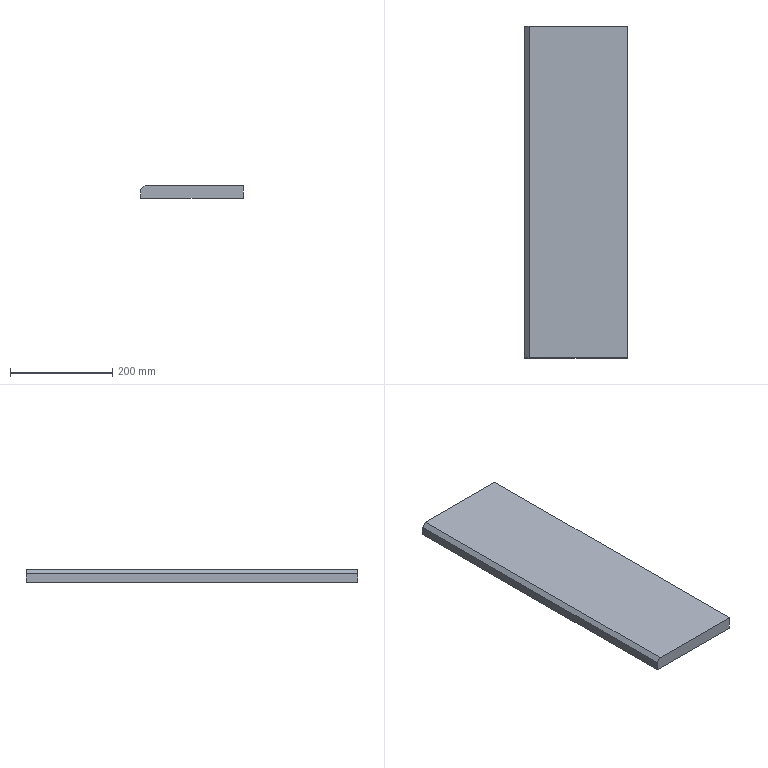Part | SolidWorks | features Chamfer 1, Extrusion 1 | 1 solid | 7 faces | box 200 x 650 x 25 mm | volume 3229200 mm3 | plane 7
STEP:
#1=CARTESIAN_POINT('',(0.,0.,17.));
#2=VERTEX_POINT('',#1);
#3=CARTESIAN_POINT('',(0.,0.,0.));
#4=VERTEX_POINT('',#3);
#5=CARTESIAN_POINT('',(0.,0.,25.));
#6=DIRECTION('',(0.,0.,-1.));
#7=VECTOR('',#6,1000.);
#8=LINE('',#5,#7);
#9=EDGE_CURVE('',#2,#4,#8,.T.);
#10=ORIENTED_EDGE('',*,*,#9,.F.);
#11=CARTESIAN_POINT('',(0.,650.,17.));
#12=VERTEX_POINT('',#11);
#13=CARTESIAN_POINT('',(0.,0.,17.));
#14=DIRECTION('',(0.,1.,0.));
#15=VECTOR('',#14,1000.);
#16=LINE('',#13,#15);
#17=EDGE_CURVE('',#2,#12,#16,.T.);
#18=ORIENTED_EDGE('',*,*,#17,.T.);
#19=CARTESIAN_POINT('',(0.,650.,0.));
#20=VERTEX_POINT('',#19);
#21=CARTESIAN_POINT('',(0.,650.,25.));
#22=DIRECTION('',(0.,0.,-1.));
#23=VECTOR('',#22,1000.);
#24=LINE('',#21,#23);
#25=EDGE_CURVE('',#12,#20,#24,.T.);
#26=ORIENTED_EDGE('',*,*,#25,.T.);
#27=CARTESIAN_POINT('',(0.,0.,0.));
#28=DIRECTION('',(0.,-1.,0.));
#29=VECTOR('',#28,1000.);
#30=LINE('',#27,#29);
#31=EDGE_CURVE('',#20,#4,#30,.T.);
#32=ORIENTED_EDGE('',*,*,#31,.T.);
#33=EDGE_LOOP('',(#10,#18,#26,#32));
#34=FACE_OUTER_BOUND('',#33,.T.);
#35=CARTESIAN_POINT('',(0.,0.,25.));
#36=DIRECTION('',(1.,0.,0.));
#37=DIRECTION('',(0.,0.,-1.));
#38=AXIS2_PLACEMENT_3D('',#35,#36,#37);
#39=PLANE('',#38);
#40=ADVANCED_FACE('',(#34),#39,.F.);
#41=CARTESIAN_POINT('',(8.,0.,25.));
#42=VERTEX_POINT('',#41);
#43=CARTESIAN_POINT('',(200.,0.,25.));
#44=VERTEX_POINT('',#43);
#45=CARTESIAN_POINT('',(0.,0.,25.));
#46=DIRECTION('',(1.,0.,0.));
#47=VECTOR('',#46,1000.);
#48=LINE('',#45,#47);
#49=EDGE_CURVE('',#42,#44,#48,.T.);
#50=ORIENTED_EDGE('',*,*,#49,.F.);
#51=CARTESIAN_POINT('',(8.,0.,25.));
#52=DIRECTION('',(-0.7071,0.,-0.7071));
#53=VECTOR('',#52,1000.);
#54=LINE('',#51,#53);
#55=EDGE_CURVE('',#42,#2,#54,.T.);
#56=ORIENTED_EDGE('',*,*,#55,.T.);
#57=ORIENTED_EDGE('',*,*,#9,.T.);
#58=CARTESIAN_POINT('',(200.,0.,0.));
#59=VERTEX_POINT('',#58);
#60=CARTESIAN_POINT('',(0.,0.,0.));
#61=DIRECTION('',(1.,0.,0.));
#62=VECTOR('',#61,1000.);
#63=LINE('',#60,#62);
#64=EDGE_CURVE('',#4,#59,#63,.T.);
#65=ORIENTED_EDGE('',*,*,#64,.T.);
#66=CARTESIAN_POINT('',(200.,0.,25.));
#67=DIRECTION('',(0.,0.,-1.));
#68=VECTOR('',#67,1000.);
#69=LINE('',#66,#68);
#70=EDGE_CURVE('',#44,#59,#69,.T.);
#71=ORIENTED_EDGE('',*,*,#70,.F.);
#72=EDGE_LOOP('',(#50,#56,#57,#65,#71));
#73=FACE_OUTER_BOUND('',#72,.T.);
#74=CARTESIAN_POINT('',(0.,0.,25.));
#75=DIRECTION('',(0.,1.,0.));
#76=DIRECTION('',(0.,0.,1.));
#77=AXIS2_PLACEMENT_3D('',#74,#75,#76);
#78=PLANE('',#77);
#79=ADVANCED_FACE('',(#73),#78,.F.);
#80=CARTESIAN_POINT('',(200.,650.,0.));
#81=VERTEX_POINT('',#80);
#82=CARTESIAN_POINT('',(200.,0.,0.));
#83=DIRECTION('',(0.,1.,0.));
#84=VECTOR('',#83,1000.);
#85=LINE('',#82,#84);
#86=EDGE_CURVE('',#59,#81,#85,.T.);
#87=ORIENTED_EDGE('',*,*,#86,.T.);
#88=CARTESIAN_POINT('',(200.,650.,25.));
#89=VERTEX_POINT('',#88);
#90=CARTESIAN_POINT('',(200.,650.,25.));
#91=DIRECTION('',(0.,0.,-1.));
#92=VECTOR('',#91,1000.);
#93=LINE('',#90,#92);
#94=EDGE_CURVE('',#89,#81,#93,.T.);
#95=ORIENTED_EDGE('',*,*,#94,.F.);
#96=CARTESIAN_POINT('',(200.,0.,25.));
#97=DIRECTION('',(0.,1.,0.));
#98=VECTOR('',#97,1000.);
#99=LINE('',#96,#98);
#100=EDGE_CURVE('',#44,#89,#99,.T.);
#101=ORIENTED_EDGE('',*,*,#100,.F.);
#102=ORIENTED_EDGE('',*,*,#70,.T.);
#103=EDGE_LOOP('',(#87,#95,#101,#102));
#104=FACE_OUTER_BOUND('',#103,.T.);
#105=CARTESIAN_POINT('',(200.,0.,25.));
#106=DIRECTION('',(-1.,0.,0.));
#107=DIRECTION('',(0.,0.,1.));
#108=AXIS2_PLACEMENT_3D('',#105,#106,#107);
#109=PLANE('',#108);
#110=ADVANCED_FACE('',(#104),#109,.F.);
#111=ORIENTED_EDGE('',*,*,#25,.F.);
#112=CARTESIAN_POINT('',(8.,650.,25.));
#113=VERTEX_POINT('',#112);
#114=CARTESIAN_POINT('',(8.,650.,25.));
#115=DIRECTION('',(0.7071,0.,0.7071));
#116=VECTOR('',#115,1000.);
#117=LINE('',#114,#116);
#118=EDGE_CURVE('',#12,#113,#117,.T.);
#119=ORIENTED_EDGE('',*,*,#118,.T.);
#120=CARTESIAN_POINT('',(0.,650.,25.));
#121=DIRECTION('',(-1.,0.,0.));
#122=VECTOR('',#121,1000.);
#123=LINE('',#120,#122);
#124=EDGE_CURVE('',#89,#113,#123,.T.);
#125=ORIENTED_EDGE('',*,*,#124,.F.);
#126=ORIENTED_EDGE('',*,*,#94,.T.);
#127=CARTESIAN_POINT('',(0.,650.,0.));
#128=DIRECTION('',(-1.,0.,0.));
#129=VECTOR('',#128,1000.);
#130=LINE('',#127,#129);
#131=EDGE_CURVE('',#81,#20,#130,.T.);
#132=ORIENTED_EDGE('',*,*,#131,.T.);
#133=EDGE_LOOP('',(#111,#119,#125,#126,#132));
#134=FACE_OUTER_BOUND('',#133,.T.);
#135=CARTESIAN_POINT('',(0.,650.,25.));
#136=DIRECTION('',(0.,-1.,0.));
#137=DIRECTION('',(0.,0.,-1.));
#138=AXIS2_PLACEMENT_3D('',#135,#136,#137);
#139=PLANE('',#138);
#140=ADVANCED_FACE('',(#134),#139,.F.);
#141=ORIENTED_EDGE('',*,*,#124,.T.);
#142=CARTESIAN_POINT('',(8.,650.,25.));
#143=DIRECTION('',(0.,-1.,0.));
#144=VECTOR('',#143,1000.);
#145=LINE('',#142,#144);
#146=EDGE_CURVE('',#113,#42,#145,.T.);
#147=ORIENTED_EDGE('',*,*,#146,.T.);
#148=ORIENTED_EDGE('',*,*,#49,.T.);
#149=ORIENTED_EDGE('',*,*,#100,.T.);
#150=EDGE_LOOP('',(#141,#147,#148,#149));
#151=FACE_OUTER_BOUND('',#150,.T.);
#152=CARTESIAN_POINT('',(0.,650.,25.));
#153=DIRECTION('',(0.,0.,-1.));
#154=DIRECTION('',(-1.,0.,0.));
#155=AXIS2_PLACEMENT_3D('',#152,#153,#154);
#156=PLANE('',#155);
#157=ADVANCED_FACE('',(#151),#156,.F.);
#158=ORIENTED_EDGE('',*,*,#31,.F.);
#159=ORIENTED_EDGE('',*,*,#131,.F.);
#160=ORIENTED_EDGE('',*,*,#86,.F.);
#161=ORIENTED_EDGE('',*,*,#64,.F.);
#162=EDGE_LOOP('',(#158,#159,#160,#161));
#163=FACE_OUTER_BOUND('',#162,.T.);
#164=CARTESIAN_POINT('',(0.,650.,0.));
#165=DIRECTION('',(0.,0.,-1.));
#166=DIRECTION('',(-1.,0.,0.));
#167=AXIS2_PLACEMENT_3D('',#164,#165,#166);
#168=PLANE('',#167);
#169=ADVANCED_FACE('',(#163),#168,.T.);
#170=ORIENTED_EDGE('',*,*,#118,.F.);
#171=ORIENTED_EDGE('',*,*,#17,.F.);
#172=ORIENTED_EDGE('',*,*,#55,.F.);
#173=ORIENTED_EDGE('',*,*,#146,.F.);
#174=EDGE_LOOP('',(#170,#171,#172,#173));
#175=FACE_OUTER_BOUND('',#174,.T.);
#176=CARTESIAN_POINT('',(8.,650.,25.));
#177=DIRECTION('',(0.7071,0.,-0.7071));
#178=DIRECTION('',(-0.7071,0.,-0.7071));
#179=AXIS2_PLACEMENT_3D('',#176,#177,#178);
#180=PLANE('',#179);
#181=ADVANCED_FACE('',(#175),#180,.F.);
#182=CLOSED_SHELL('',(#40,#79,#110,#140,#157,#169,#181));
#183=MANIFOLD_SOLID_BREP('',#182);
#184=CARTESIAN_POINT('',(0.,0.,0.));
#185=DIRECTION('',(0.,0.,1.));
#186=DIRECTION('',(1.,0.,0.));
#187=AXIS2_PLACEMENT_3D('',#184,#185,#186);
#188=(LENGTH_UNIT()NAMED_UNIT(*)SI_UNIT(.MILLI.,.METRE.));
#189=UNCERTAINTY_MEASURE_WITH_UNIT(LENGTH_MEASURE(0.00001),#188,'','');
#190=(NAMED_UNIT(*)PLANE_ANGLE_UNIT()SI_UNIT($,.RADIAN.));
#191=(NAMED_UNIT(*)SI_UNIT($,.STERADIAN.)SOLID_ANGLE_UNIT());
#192=(GEOMETRIC_REPRESENTATION_CONTEXT(3)GLOBAL_UNCERTAINTY_ASSIGNED_CONTEXT((#189))GLOBAL_UNIT_ASSIGNED_CONTEXT((#188,#190,#191))REPRESENTATION_CONTEXT('',''));
#193=ADVANCED_BREP_SHAPE_REPRESENTATION('',(#183,#187),#192);